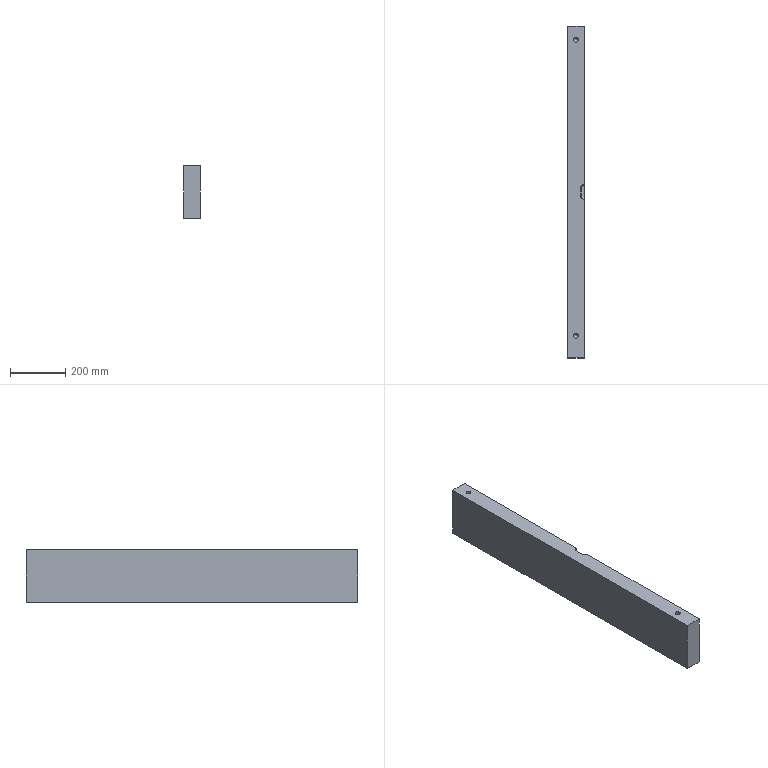Part | STEP file | lll_id4458_x_t | 1 solid | 25 faces | box 60 x 1200 x 190 mm | volume 13623980 mm3 | plane 10 | cylinder 9 | cone 4 | sphere 2 | commonest cylinder face diameters 20 x5 17.505 x2 17.506 x2
STEP:
#1=CARTESIAN_POINT('',(855.188,550.,-370.));
#2=VERTEX_POINT('',#1);
#3=CARTESIAN_POINT('',(846.435,550.,-370.));
#4=DIRECTION('',(0.,0.,1.));
#5=DIRECTION('',(1.,0.,0.));
#6=AXIS2_PLACEMENT_3D('',#3,#4,#5);
#7=CIRCLE('',#6,8.752);
#8=EDGE_CURVE('',#2,#2,#7,.T.);
#9=ORIENTED_EDGE('',*,*,#8,.T.);
#10=EDGE_LOOP('',(#9));
#11=FACE_BOUND('',#10,.T.);
#12=CARTESIAN_POINT('',(876.435,600.,-370.));
#13=VERTEX_POINT('',#12);
#14=CARTESIAN_POINT('',(876.435,-600.,-370.));
#15=VERTEX_POINT('',#14);
#16=CARTESIAN_POINT('',(876.435,600.,-370.));
#17=DIRECTION('',(0.,-1.,0.));
#18=VECTOR('',#17,1.);
#19=LINE('',#16,#18);
#20=EDGE_CURVE('',#13,#15,#19,.T.);
#21=ORIENTED_EDGE('',*,*,#20,.T.);
#22=CARTESIAN_POINT('',(816.435,-600.,-370.));
#23=VERTEX_POINT('',#22);
#24=CARTESIAN_POINT('',(876.435,-600.,-370.));
#25=DIRECTION('',(-1.,0.,0.));
#26=VECTOR('',#25,1.);
#27=LINE('',#24,#26);
#28=EDGE_CURVE('',#15,#23,#27,.T.);
#29=ORIENTED_EDGE('',*,*,#28,.T.);
#30=CARTESIAN_POINT('',(816.435,600.,-370.));
#31=VERTEX_POINT('',#30);
#32=CARTESIAN_POINT('',(816.435,1.,-370.));
#33=DIRECTION('',(0.,-1.,0.));
#34=VECTOR('',#33,1.);
#35=LINE('',#32,#34);
#36=EDGE_CURVE('',#31,#23,#35,.T.);
#37=ORIENTED_EDGE('',*,*,#36,.F.);
#38=CARTESIAN_POINT('',(-3093.565,600.,-370.));
#39=DIRECTION('',(1.,0.,0.));
#40=VECTOR('',#39,1.);
#41=LINE('',#38,#40);
#42=EDGE_CURVE('',#31,#13,#41,.T.);
#43=ORIENTED_EDGE('',*,*,#42,.T.);
#44=EDGE_LOOP('',(#21,#29,#37,#43));
#45=FACE_BOUND('',#44,.T.);
#46=CARTESIAN_POINT('',(855.188,-520.,-370.));
#47=VERTEX_POINT('',#46);
#48=CARTESIAN_POINT('',(846.435,-520.,-370.));
#49=DIRECTION('',(0.,0.,1.));
#50=DIRECTION('',(1.,0.,0.));
#51=AXIS2_PLACEMENT_3D('',#48,#49,#50);
#52=CIRCLE('',#51,8.752);
#53=EDGE_CURVE('',#47,#47,#52,.T.);
#54=ORIENTED_EDGE('',*,*,#53,.T.);
#55=EDGE_LOOP('',(#54));
#56=FACE_BOUND('',#55,.T.);
#57=CARTESIAN_POINT('',(3062.751,1.,-370.));
#58=DIRECTION('',(0.,0.,-1.));
#59=DIRECTION('',(-1.,0.,0.));
#60=AXIS2_PLACEMENT_3D('',#57,#58,#59);
#61=PLANE('',#60);
#62=ADVANCED_FACE('',(#11,#45,#56),#61,.T.);
#63=CARTESIAN_POINT('',(876.435,25.5,-180.));
#64=VERTEX_POINT('',#63);
#65=CARTESIAN_POINT('',(876.435,25.5,-194.289));
#66=VERTEX_POINT('',#65);
#67=CARTESIAN_POINT('',(876.435,25.5,-251.25));
#68=DIRECTION('',(0.,0.,-1.));
#69=VECTOR('',#68,1.);
#70=LINE('',#67,#69);
#71=EDGE_CURVE('',#64,#66,#70,.T.);
#72=ORIENTED_EDGE('',*,*,#71,.T.);
#73=CARTESIAN_POINT('',(876.435,15.5,-208.431));
#74=VERTEX_POINT('',#73);
#75=CARTESIAN_POINT('',(876.435,15.5,-194.289));
#76=DIRECTION('',(-1.,0.,0.));
#77=DIRECTION('',(0.,0.,1.));
#78=AXIS2_PLACEMENT_3D('',#75,#76,#77);
#79=ELLIPSE('',#78,14.142,10.);
#80=EDGE_CURVE('',#66,#74,#79,.T.);
#81=ORIENTED_EDGE('',*,*,#80,.T.);
#82=CARTESIAN_POINT('',(876.435,-15.5,-208.431));
#83=VERTEX_POINT('',#82);
#84=CARTESIAN_POINT('',(876.435,-204.288,-208.431));
#85=DIRECTION('',(0.,-1.,0.));
#86=VECTOR('',#85,1.);
#87=LINE('',#84,#86);
#88=EDGE_CURVE('',#74,#83,#87,.T.);
#89=ORIENTED_EDGE('',*,*,#88,.T.);
#90=CARTESIAN_POINT('',(876.435,-25.5,-194.289));
#91=VERTEX_POINT('',#90);
#92=CARTESIAN_POINT('',(876.435,-15.5,-194.289));
#93=DIRECTION('',(-1.,0.,0.));
#94=DIRECTION('',(0.,0.,-1.));
#95=AXIS2_PLACEMENT_3D('',#92,#93,#94);
#96=ELLIPSE('',#95,14.142,10.);
#97=EDGE_CURVE('',#83,#91,#96,.T.);
#98=ORIENTED_EDGE('',*,*,#97,.T.);
#99=CARTESIAN_POINT('',(876.435,-25.5,-180.));
#100=VERTEX_POINT('',#99);
#101=CARTESIAN_POINT('',(876.435,-25.5,-251.25));
#102=DIRECTION('',(0.,0.,1.));
#103=VECTOR('',#102,1.);
#104=LINE('',#101,#103);
#105=EDGE_CURVE('',#91,#100,#104,.T.);
#106=ORIENTED_EDGE('',*,*,#105,.T.);
#107=CARTESIAN_POINT('',(876.435,-600.,-180.));
#108=VERTEX_POINT('',#107);
#109=CARTESIAN_POINT('',(876.435,1.,-180.));
#110=DIRECTION('',(0.,-1.,0.));
#111=VECTOR('',#110,1.);
#112=LINE('',#109,#111);
#113=EDGE_CURVE('',#100,#108,#112,.T.);
#114=ORIENTED_EDGE('',*,*,#113,.T.);
#115=CARTESIAN_POINT('',(876.435,-600.,-182.5));
#116=DIRECTION('',(0.,0.,-1.));
#117=VECTOR('',#116,1.);
#118=LINE('',#115,#117);
#119=EDGE_CURVE('',#108,#15,#118,.T.);
#120=ORIENTED_EDGE('',*,*,#119,.T.);
#121=ORIENTED_EDGE('',*,*,#20,.F.);
#122=CARTESIAN_POINT('',(876.435,600.,-180.));
#123=VERTEX_POINT('',#122);
#124=CARTESIAN_POINT('',(876.435,600.,-182.5));
#125=DIRECTION('',(0.,0.,-1.));
#126=VECTOR('',#125,1.);
#127=LINE('',#124,#126);
#128=EDGE_CURVE('',#123,#13,#127,.T.);
#129=ORIENTED_EDGE('',*,*,#128,.F.);
#130=CARTESIAN_POINT('',(876.435,1.,-180.));
#131=DIRECTION('',(0.,-1.,0.));
#132=VECTOR('',#131,1.);
#133=LINE('',#130,#132);
#134=EDGE_CURVE('',#123,#64,#133,.T.);
#135=ORIENTED_EDGE('',*,*,#134,.T.);
#136=EDGE_LOOP('',(#72,#81,#89,#98,#106,#114,#120,#121,#129,#135));
#137=FACE_OUTER_BOUND('',#136,.T.);
#138=CARTESIAN_POINT('',(876.435,600.,-182.5));
#139=DIRECTION('',(1.,0.,0.));
#140=DIRECTION('',(0.,0.,-1.));
#141=AXIS2_PLACEMENT_3D('',#138,#139,#140);
#142=PLANE('',#141);
#143=ADVANCED_FACE('',(#137),#142,.T.);
#144=CARTESIAN_POINT('',(816.435,-600.,-180.));
#145=VERTEX_POINT('',#144);
#146=CARTESIAN_POINT('',(816.435,-600.,-182.5));
#147=DIRECTION('',(0.,0.,-1.));
#148=VECTOR('',#147,1.);
#149=LINE('',#146,#148);
#150=EDGE_CURVE('',#145,#23,#149,.T.);
#151=ORIENTED_EDGE('',*,*,#150,.T.);
#152=ORIENTED_EDGE('',*,*,#28,.F.);
#153=ORIENTED_EDGE('',*,*,#119,.F.);
#154=CARTESIAN_POINT('',(3062.751,-600.,-180.));
#155=DIRECTION('',(-1.,0.,0.));
#156=VECTOR('',#155,1.);
#157=LINE('',#154,#156);
#158=EDGE_CURVE('',#108,#145,#157,.T.);
#159=ORIENTED_EDGE('',*,*,#158,.T.);
#160=EDGE_LOOP('',(#151,#152,#153,#159));
#161=FACE_OUTER_BOUND('',#160,.T.);
#162=CARTESIAN_POINT('',(876.435,-600.,-182.5));
#163=DIRECTION('',(0.,-1.,0.));
#164=DIRECTION('',(0.,0.,-1.));
#165=AXIS2_PLACEMENT_3D('',#162,#163,#164);
#166=PLANE('',#165);
#167=ADVANCED_FACE('',(#161),#166,.T.);
#168=CARTESIAN_POINT('',(816.435,600.,-180.));
#169=VERTEX_POINT('',#168);
#170=CARTESIAN_POINT('',(816.435,600.,-182.5));
#171=DIRECTION('',(0.,0.,1.));
#172=VECTOR('',#171,1.);
#173=LINE('',#170,#172);
#174=EDGE_CURVE('',#31,#169,#173,.T.);
#175=ORIENTED_EDGE('',*,*,#174,.T.);
#176=CARTESIAN_POINT('',(3062.751,600.,-180.));
#177=DIRECTION('',(1.,0.,0.));
#178=VECTOR('',#177,1.);
#179=LINE('',#176,#178);
#180=EDGE_CURVE('',#169,#123,#179,.T.);
#181=ORIENTED_EDGE('',*,*,#180,.T.);
#182=ORIENTED_EDGE('',*,*,#128,.T.);
#183=ORIENTED_EDGE('',*,*,#42,.F.);
#184=EDGE_LOOP('',(#175,#181,#182,#183));
#185=FACE_OUTER_BOUND('',#184,.T.);
#186=CARTESIAN_POINT('',(-3093.565,600.,-182.5));
#187=DIRECTION('',(0.,1.,0.));
#188=DIRECTION('',(0.,0.,1.));
#189=AXIS2_PLACEMENT_3D('',#186,#187,#188);
#190=PLANE('',#189);
#191=ADVANCED_FACE('',(#185),#190,.T.);
#192=CARTESIAN_POINT('',(837.682,550.,-180.));
#193=VERTEX_POINT('',#192);
#194=CARTESIAN_POINT('',(846.435,550.,-180.));
#195=DIRECTION('',(0.,0.,-1.));
#196=DIRECTION('',(-1.,0.,0.));
#197=AXIS2_PLACEMENT_3D('',#194,#195,#196);
#198=CIRCLE('',#197,8.753);
#199=EDGE_CURVE('',#193,#193,#198,.T.);
#200=ORIENTED_EDGE('',*,*,#199,.T.);
#201=EDGE_LOOP('',(#200));
#202=FACE_BOUND('',#201,.T.);
#203=CARTESIAN_POINT('',(837.682,-520.,-180.));
#204=VERTEX_POINT('',#203);
#205=CARTESIAN_POINT('',(846.435,-520.,-180.));
#206=DIRECTION('',(0.,0.,-1.));
#207=DIRECTION('',(-1.,0.,0.));
#208=AXIS2_PLACEMENT_3D('',#205,#206,#207);
#209=CIRCLE('',#208,8.753);
#210=EDGE_CURVE('',#204,#204,#209,.T.);
#211=ORIENTED_EDGE('',*,*,#210,.T.);
#212=EDGE_LOOP('',(#211));
#213=FACE_BOUND('',#212,.T.);
#214=CARTESIAN_POINT('',(873.004,25.5,-180.));
#215=VERTEX_POINT('',#214);
#216=CARTESIAN_POINT('',(863.004,15.5,-180.));
#217=VERTEX_POINT('',#216);
#218=CARTESIAN_POINT('',(873.004,15.5,-180.));
#219=DIRECTION('',(0.,0.,1.));
#220=DIRECTION('',(1.,0.,0.));
#221=AXIS2_PLACEMENT_3D('',#218,#219,#220);
#222=CIRCLE('',#221,10.);
#223=EDGE_CURVE('',#215,#217,#222,.T.);
#224=ORIENTED_EDGE('',*,*,#223,.F.);
#225=CARTESIAN_POINT('',(898.504,25.5,-180.));
#226=DIRECTION('',(-1.,0.,0.));
#227=VECTOR('',#226,1.);
#228=LINE('',#225,#227);
#229=EDGE_CURVE('',#64,#215,#228,.T.);
#230=ORIENTED_EDGE('',*,*,#229,.F.);
#231=ORIENTED_EDGE('',*,*,#134,.F.);
#232=ORIENTED_EDGE('',*,*,#180,.F.);
#233=CARTESIAN_POINT('',(816.435,0.,-180.));
#234=DIRECTION('',(0.,1.,0.));
#235=VECTOR('',#234,1.);
#236=LINE('',#233,#235);
#237=EDGE_CURVE('',#145,#169,#236,.T.);
#238=ORIENTED_EDGE('',*,*,#237,.F.);
#239=ORIENTED_EDGE('',*,*,#158,.F.);
#240=ORIENTED_EDGE('',*,*,#113,.F.);
#241=CARTESIAN_POINT('',(873.004,-25.5,-180.));
#242=VERTEX_POINT('',#241);
#243=CARTESIAN_POINT('',(898.504,-25.5,-180.));
#244=DIRECTION('',(1.,0.,0.));
#245=VECTOR('',#244,1.);
#246=LINE('',#243,#245);
#247=EDGE_CURVE('',#242,#100,#246,.T.);
#248=ORIENTED_EDGE('',*,*,#247,.F.);
#249=CARTESIAN_POINT('',(863.004,-15.5,-180.));
#250=VERTEX_POINT('',#249);
#251=CARTESIAN_POINT('',(873.004,-15.5,-180.));
#252=DIRECTION('',(0.,0.,1.));
#253=DIRECTION('',(1.,0.,0.));
#254=AXIS2_PLACEMENT_3D('',#251,#252,#253);
#255=CIRCLE('',#254,10.);
#256=EDGE_CURVE('',#250,#242,#255,.T.);
#257=ORIENTED_EDGE('',*,*,#256,.F.);
#258=CARTESIAN_POINT('',(863.004,0.,-180.));
#259=DIRECTION('',(0.,-1.,0.));
#260=VECTOR('',#259,1.);
#261=LINE('',#258,#260);
#262=EDGE_CURVE('',#217,#250,#261,.T.);
#263=ORIENTED_EDGE('',*,*,#262,.F.);
#264=EDGE_LOOP('',(#224,#230,#231,#232,#238,#239,#240,#248,#257,#263));
#265=FACE_BOUND('',#264,.T.);
#266=CARTESIAN_POINT('',(3062.751,1.,-180.));
#267=DIRECTION('',(0.,0.,-1.));
#268=DIRECTION('',(-1.,0.,0.));
#269=AXIS2_PLACEMENT_3D('',#266,#267,#268);
#270=PLANE('',#269);
#271=ADVANCED_FACE('',(#202,#213,#265),#270,.F.);
#272=ORIENTED_EDGE('',*,*,#174,.F.);
#273=ORIENTED_EDGE('',*,*,#36,.T.);
#274=ORIENTED_EDGE('',*,*,#150,.F.);
#275=ORIENTED_EDGE('',*,*,#237,.T.);
#276=EDGE_LOOP('',(#272,#273,#274,#275));
#277=FACE_OUTER_BOUND('',#276,.T.);
#278=CARTESIAN_POINT('',(816.435,0.,-251.25));
#279=DIRECTION('',(1.,0.,0.));
#280=DIRECTION('',(0.,0.,-1.));
#281=AXIS2_PLACEMENT_3D('',#278,#279,#280);
#282=PLANE('',#281);
#283=ADVANCED_FACE('',(#277),#282,.F.);
#284=ORIENTED_EDGE('',*,*,#88,.F.);
#285=CARTESIAN_POINT('',(865.933,15.5,-197.929));
#286=VERTEX_POINT('',#285);
#287=CARTESIAN_POINT('',(876.435,15.5,-208.431));
#288=DIRECTION('',(0.7071,0.,-0.7071));
#289=VECTOR('',#288,1.);
#290=LINE('',#287,#289);
#291=EDGE_CURVE('',#286,#74,#290,.T.);
#292=ORIENTED_EDGE('',*,*,#291,.F.);
#293=CARTESIAN_POINT('',(865.933,-15.5,-197.929));
#294=VERTEX_POINT('',#293);
#295=CARTESIAN_POINT('',(865.933,35.5,-197.929));
#296=DIRECTION('',(0.,1.,0.));
#297=VECTOR('',#296,1.);
#298=LINE('',#295,#297);
#299=EDGE_CURVE('',#294,#286,#298,.T.);
#300=ORIENTED_EDGE('',*,*,#299,.F.);
#301=CARTESIAN_POINT('',(863.004,-15.5,-195.));
#302=DIRECTION('',(-0.7071,0.,0.7071));
#303=VECTOR('',#302,1.);
#304=LINE('',#301,#303);
#305=EDGE_CURVE('',#83,#294,#304,.T.);
#306=ORIENTED_EDGE('',*,*,#305,.F.);
#307=EDGE_LOOP('',(#284,#292,#300,#306));
#308=FACE_OUTER_BOUND('',#307,.T.);
#309=CARTESIAN_POINT('',(863.004,0.,-195.));
#310=DIRECTION('',(0.7071,0.,0.7071));
#311=DIRECTION('',(0.,1.,0.));
#312=AXIS2_PLACEMENT_3D('',#309,#310,#311);
#313=PLANE('',#312);
#314=ADVANCED_FACE('',(#308),#313,.T.);
#315=ORIENTED_EDGE('',*,*,#223,.T.);
#316=CARTESIAN_POINT('',(863.004,15.5,-190.858));
#317=VERTEX_POINT('',#316);
#318=CARTESIAN_POINT('',(863.004,15.5,-195.));
#319=DIRECTION('',(0.,0.,-1.));
#320=VECTOR('',#319,1.);
#321=LINE('',#318,#320);
#322=EDGE_CURVE('',#217,#317,#321,.T.);
#323=ORIENTED_EDGE('',*,*,#322,.T.);
#324=CARTESIAN_POINT('',(873.004,25.5,-190.858));
#325=VERTEX_POINT('',#324);
#326=CARTESIAN_POINT('',(873.004,15.5,-190.858));
#327=DIRECTION('',(0.,0.,-1.));
#328=DIRECTION('',(-1.,0.,0.));
#329=AXIS2_PLACEMENT_3D('',#326,#327,#328);
#330=CIRCLE('',#329,10.);
#331=EDGE_CURVE('',#317,#325,#330,.T.);
#332=ORIENTED_EDGE('',*,*,#331,.T.);
#333=CARTESIAN_POINT('',(873.004,25.5,-180.));
#334=DIRECTION('',(0.,0.,1.));
#335=VECTOR('',#334,1.);
#336=LINE('',#333,#335);
#337=EDGE_CURVE('',#325,#215,#336,.T.);
#338=ORIENTED_EDGE('',*,*,#337,.T.);
#339=EDGE_LOOP('',(#315,#323,#332,#338));
#340=FACE_OUTER_BOUND('',#339,.T.);
#341=CARTESIAN_POINT('',(873.004,15.5,-210.));
#342=DIRECTION('',(0.,0.,1.));
#343=DIRECTION('',(-1.,0.,0.));
#344=AXIS2_PLACEMENT_3D('',#341,#342,#343);
#345=CYLINDRICAL_SURFACE('',#344,10.);
#346=ADVANCED_FACE('',(#340),#345,.F.);
#347=ORIENTED_EDGE('',*,*,#80,.F.);
#348=CARTESIAN_POINT('',(870.075,25.5,-187.929));
#349=DIRECTION('',(-0.7071,0.,0.7071));
#350=VECTOR('',#349,1.);
#351=LINE('',#348,#350);
#352=EDGE_CURVE('',#66,#325,#351,.T.);
#353=ORIENTED_EDGE('',*,*,#352,.T.);
#354=CARTESIAN_POINT('',(873.004,15.5,-190.858));
#355=DIRECTION('',(-0.7071,0.,0.7071));
#356=DIRECTION('',(-0.7071,0.,-0.7071));
#357=AXIS2_PLACEMENT_3D('',#354,#355,#356);
#358=CIRCLE('',#357,10.);
#359=EDGE_CURVE('',#325,#286,#358,.T.);
#360=ORIENTED_EDGE('',*,*,#359,.T.);
#361=ORIENTED_EDGE('',*,*,#291,.T.);
#362=EDGE_LOOP('',(#347,#353,#360,#361));
#363=FACE_OUTER_BOUND('',#362,.T.);
#364=CARTESIAN_POINT('',(895.325,15.5,-213.179));
#365=DIRECTION('',(-0.7071,0.,0.7071));
#366=DIRECTION('',(-0.7071,0.,-0.7071));
#367=AXIS2_PLACEMENT_3D('',#364,#365,#366);
#368=CYLINDRICAL_SURFACE('',#367,10.);
#369=ADVANCED_FACE('',(#363),#368,.F.);
#370=CARTESIAN_POINT('',(873.004,15.5,-190.858));
#371=DIRECTION('',(0.,-1.,0.));
#372=DIRECTION('',(0.,0.,-1.));
#373=AXIS2_PLACEMENT_3D('',#370,#371,#372);
#374=CIRCLE('',#373,10.);
#375=EDGE_CURVE('',#317,#286,#374,.T.);
#376=ORIENTED_EDGE('',*,*,#375,.F.);
#377=CARTESIAN_POINT('',(863.004,-15.5,-190.858));
#378=VERTEX_POINT('',#377);
#379=CARTESIAN_POINT('',(863.004,-35.5,-190.858));
#380=DIRECTION('',(0.,-1.,0.));
#381=VECTOR('',#380,1.);
#382=LINE('',#379,#381);
#383=EDGE_CURVE('',#317,#378,#382,.T.);
#384=ORIENTED_EDGE('',*,*,#383,.T.);
#385=CARTESIAN_POINT('',(873.004,-15.5,-190.858));
#386=DIRECTION('',(0.,-1.,0.));
#387=DIRECTION('',(0.,0.,-1.));
#388=AXIS2_PLACEMENT_3D('',#385,#386,#387);
#389=CIRCLE('',#388,10.);
#390=EDGE_CURVE('',#378,#294,#389,.T.);
#391=ORIENTED_EDGE('',*,*,#390,.T.);
#392=ORIENTED_EDGE('',*,*,#299,.T.);
#393=EDGE_LOOP('',(#376,#384,#391,#392));
#394=FACE_OUTER_BOUND('',#393,.T.);
#395=CARTESIAN_POINT('',(873.004,0.,-190.858));
#396=DIRECTION('',(0.,-1.,0.));
#397=DIRECTION('',(0.,0.,-1.));
#398=AXIS2_PLACEMENT_3D('',#395,#396,#397);
#399=CYLINDRICAL_SURFACE('',#398,10.);
#400=ADVANCED_FACE('',(#394),#399,.F.);
#401=ORIENTED_EDGE('',*,*,#331,.F.);
#402=ORIENTED_EDGE('',*,*,#375,.T.);
#403=ORIENTED_EDGE('',*,*,#359,.F.);
#404=EDGE_LOOP('',(#401,#402,#403));
#405=FACE_OUTER_BOUND('',#404,.T.);
#406=CARTESIAN_POINT('',(873.004,15.5,-190.858));
#407=DIRECTION('',(0.,0.,1.));
#408=DIRECTION('',(-1.,0.,0.));
#409=AXIS2_PLACEMENT_3D('',#406,#407,#408);
#410=SPHERICAL_SURFACE('',#409,10.);
#411=ADVANCED_FACE('',(#405),#410,.F.);
#412=ORIENTED_EDGE('',*,*,#256,.T.);
#413=CARTESIAN_POINT('',(873.004,-25.5,-190.858));
#414=VERTEX_POINT('',#413);
#415=CARTESIAN_POINT('',(873.004,-25.5,-195.));
#416=DIRECTION('',(0.,0.,-1.));
#417=VECTOR('',#416,1.);
#418=LINE('',#415,#417);
#419=EDGE_CURVE('',#242,#414,#418,.T.);
#420=ORIENTED_EDGE('',*,*,#419,.T.);
#421=CARTESIAN_POINT('',(873.004,-15.5,-190.858));
#422=DIRECTION('',(0.,0.,-1.));
#423=DIRECTION('',(-1.,0.,0.));
#424=AXIS2_PLACEMENT_3D('',#421,#422,#423);
#425=CIRCLE('',#424,10.);
#426=EDGE_CURVE('',#414,#378,#425,.T.);
#427=ORIENTED_EDGE('',*,*,#426,.T.);
#428=CARTESIAN_POINT('',(863.004,-15.5,-180.));
#429=DIRECTION('',(0.,0.,1.));
#430=VECTOR('',#429,1.);
#431=LINE('',#428,#430);
#432=EDGE_CURVE('',#378,#250,#431,.T.);
#433=ORIENTED_EDGE('',*,*,#432,.T.);
#434=EDGE_LOOP('',(#412,#420,#427,#433));
#435=FACE_OUTER_BOUND('',#434,.T.);
#436=CARTESIAN_POINT('',(873.004,-15.5,-210.));
#437=DIRECTION('',(0.,0.,1.));
#438=DIRECTION('',(-1.,0.,0.));
#439=AXIS2_PLACEMENT_3D('',#436,#437,#438);
#440=CYLINDRICAL_SURFACE('',#439,10.);
#441=ADVANCED_FACE('',(#435),#440,.F.);
#442=ORIENTED_EDGE('',*,*,#426,.F.);
#443=CARTESIAN_POINT('',(873.004,-15.5,-190.858));
#444=DIRECTION('',(0.7071,0.,-0.7071));
#445=DIRECTION('',(0.7071,0.,0.7071));
#446=AXIS2_PLACEMENT_3D('',#443,#444,#445);
#447=CIRCLE('',#446,10.);
#448=EDGE_CURVE('',#414,#294,#447,.T.);
#449=ORIENTED_EDGE('',*,*,#448,.T.);
#450=ORIENTED_EDGE('',*,*,#390,.F.);
#451=EDGE_LOOP('',(#442,#449,#450));
#452=FACE_OUTER_BOUND('',#451,.T.);
#453=CARTESIAN_POINT('',(873.004,-15.5,-190.858));
#454=DIRECTION('',(0.,0.,1.));
#455=DIRECTION('',(-1.,0.,0.));
#456=AXIS2_PLACEMENT_3D('',#453,#454,#455);
#457=SPHERICAL_SURFACE('',#456,10.);
#458=ADVANCED_FACE('',(#452),#457,.F.);
#459=ORIENTED_EDGE('',*,*,#448,.F.);
#460=CARTESIAN_POINT('',(883.506,-25.5,-201.36));
#461=DIRECTION('',(0.7071,0.,-0.7071));
#462=VECTOR('',#461,1.);
#463=LINE('',#460,#462);
#464=EDGE_CURVE('',#414,#91,#463,.T.);
#465=ORIENTED_EDGE('',*,*,#464,.T.);
#466=ORIENTED_EDGE('',*,*,#97,.F.);
#467=ORIENTED_EDGE('',*,*,#305,.T.);
#468=EDGE_LOOP('',(#459,#465,#466,#467));
#469=FACE_OUTER_BOUND('',#468,.T.);
#470=CARTESIAN_POINT('',(895.325,-15.5,-213.179));
#471=DIRECTION('',(0.7071,0.,-0.7071));
#472=DIRECTION('',(0.7071,0.,0.7071));
#473=AXIS2_PLACEMENT_3D('',#470,#471,#472);
#474=CYLINDRICAL_SURFACE('',#473,10.);
#475=ADVANCED_FACE('',(#469),#474,.F.);
#476=ORIENTED_EDGE('',*,*,#352,.F.);
#477=ORIENTED_EDGE('',*,*,#71,.F.);
#478=ORIENTED_EDGE('',*,*,#229,.T.);
#479=ORIENTED_EDGE('',*,*,#337,.F.);
#480=EDGE_LOOP('',(#476,#477,#478,#479));
#481=FACE_OUTER_BOUND('',#480,.T.);
#482=CARTESIAN_POINT('',(898.504,25.5,-210.));
#483=DIRECTION('',(0.,1.,0.));
#484=DIRECTION('',(0.,0.,1.));
#485=AXIS2_PLACEMENT_3D('',#482,#483,#484);
#486=PLANE('',#485);
#487=ADVANCED_FACE('',(#481),#486,.F.);
#488=ORIENTED_EDGE('',*,*,#419,.F.);
#489=ORIENTED_EDGE('',*,*,#247,.T.);
#490=ORIENTED_EDGE('',*,*,#105,.F.);
#491=ORIENTED_EDGE('',*,*,#464,.F.);
#492=EDGE_LOOP('',(#488,#489,#490,#491));
#493=FACE_OUTER_BOUND('',#492,.T.);
#494=CARTESIAN_POINT('',(898.504,-25.5,-210.));
#495=DIRECTION('',(0.,-1.,0.));
#496=DIRECTION('',(0.,0.,-1.));
#497=AXIS2_PLACEMENT_3D('',#494,#495,#496);
#498=PLANE('',#497);
#499=ADVANCED_FACE('',(#493),#498,.F.);
#500=ORIENTED_EDGE('',*,*,#383,.F.);
#501=ORIENTED_EDGE('',*,*,#322,.F.);
#502=ORIENTED_EDGE('',*,*,#262,.T.);
#503=ORIENTED_EDGE('',*,*,#432,.F.);
#504=EDGE_LOOP('',(#500,#501,#502,#503));
#505=FACE_OUTER_BOUND('',#504,.T.);
#506=CARTESIAN_POINT('',(863.004,0.,-210.));
#507=DIRECTION('',(-1.,0.,0.));
#508=DIRECTION('',(0.,0.,-1.));
#509=AXIS2_PLACEMENT_3D('',#506,#507,#508);
#510=PLANE('',#509);
#511=ADVANCED_FACE('',(#505),#510,.F.);
#512=CARTESIAN_POINT('',(855.188,550.,-328.747));
#513=VERTEX_POINT('',#512);
#514=CARTESIAN_POINT('',(846.435,550.,-328.747));
#515=DIRECTION('',(0.,0.,1.));
#516=DIRECTION('',(1.,0.,0.));
#517=AXIS2_PLACEMENT_3D('',#514,#515,#516);
#518=CIRCLE('',#517,8.752);
#519=EDGE_CURVE('',#513,#513,#518,.T.);
#520=ORIENTED_EDGE('',*,*,#519,.T.);
#521=EDGE_LOOP('',(#520));
#522=FACE_BOUND('',#521,.T.);
#523=ORIENTED_EDGE('',*,*,#8,.F.);
#524=EDGE_LOOP('',(#523));
#525=FACE_BOUND('',#524,.T.);
#526=CARTESIAN_POINT('',(846.435,550.,-370.));
#527=DIRECTION('',(0.,0.,1.));
#528=DIRECTION('',(-1.,0.,0.));
#529=AXIS2_PLACEMENT_3D('',#526,#527,#528);
#530=CYLINDRICAL_SURFACE('',#529,8.752);
#531=ADVANCED_FACE('',(#522,#525),#530,.F.);
#532=CARTESIAN_POINT('',(846.435,550.,-319.994));
#533=VERTEX_POINT('',#532);
#534=VERTEX_LOOP('',#533);
#535=FACE_BOUND('',#534,.T.);
#536=ORIENTED_EDGE('',*,*,#519,.F.);
#537=EDGE_LOOP('',(#536));
#538=FACE_BOUND('',#537,.T.);
#539=CARTESIAN_POINT('',(846.435,550.,-328.747));
#540=DIRECTION('',(0.,0.,-1.));
#541=DIRECTION('',(1.,0.,0.));
#542=AXIS2_PLACEMENT_3D('',#539,#540,#541);
#543=CONICAL_SURFACE('',#542,8.752,45.);
#544=ADVANCED_FACE('',(#535,#538),#543,.F.);
#545=CARTESIAN_POINT('',(855.188,-520.,-328.747));
#546=VERTEX_POINT('',#545);
#547=CARTESIAN_POINT('',(846.435,-520.,-328.747));
#548=DIRECTION('',(0.,0.,1.));
#549=DIRECTION('',(1.,0.,0.));
#550=AXIS2_PLACEMENT_3D('',#547,#548,#549);
#551=CIRCLE('',#550,8.752);
#552=EDGE_CURVE('',#546,#546,#551,.T.);
#553=ORIENTED_EDGE('',*,*,#552,.T.);
#554=EDGE_LOOP('',(#553));
#555=FACE_BOUND('',#554,.T.);
#556=ORIENTED_EDGE('',*,*,#53,.F.);
#557=EDGE_LOOP('',(#556));
#558=FACE_BOUND('',#557,.T.);
#559=CARTESIAN_POINT('',(846.435,-520.,-370.));
#560=DIRECTION('',(0.,0.,1.));
#561=DIRECTION('',(-1.,0.,0.));
#562=AXIS2_PLACEMENT_3D('',#559,#560,#561);
#563=CYLINDRICAL_SURFACE('',#562,8.752);
#564=ADVANCED_FACE('',(#555,#558),#563,.F.);
#565=CARTESIAN_POINT('',(846.435,-520.,-319.994));
#566=VERTEX_POINT('',#565);
#567=VERTEX_LOOP('',#566);
#568=FACE_BOUND('',#567,.T.);
#569=ORIENTED_EDGE('',*,*,#552,.F.);
#570=EDGE_LOOP('',(#569));
#571=FACE_BOUND('',#570,.T.);
#572=CARTESIAN_POINT('',(846.435,-520.,-328.747));
#573=DIRECTION('',(0.,0.,-1.));
#574=DIRECTION('',(1.,0.,0.));
#575=AXIS2_PLACEMENT_3D('',#572,#573,#574);
#576=CONICAL_SURFACE('',#575,8.752,45.);
#577=ADVANCED_FACE('',(#568,#571),#576,.F.);
#578=CARTESIAN_POINT('',(837.682,-520.,-221.253));
#579=VERTEX_POINT('',#578);
#580=CARTESIAN_POINT('',(846.435,-520.,-221.253));
#581=DIRECTION('',(0.,0.,-1.));
#582=DIRECTION('',(-1.,0.,0.));
#583=AXIS2_PLACEMENT_3D('',#580,#581,#582);
#584=CIRCLE('',#583,8.753);
#585=EDGE_CURVE('',#579,#579,#584,.T.);
#586=ORIENTED_EDGE('',*,*,#585,.T.);
#587=EDGE_LOOP('',(#586));
#588=FACE_BOUND('',#587,.T.);
#589=ORIENTED_EDGE('',*,*,#210,.F.);
#590=EDGE_LOOP('',(#589));
#591=FACE_BOUND('',#590,.T.);
#592=CARTESIAN_POINT('',(846.435,-520.,-180.));
#593=DIRECTION('',(0.,0.,-1.));
#594=DIRECTION('',(1.,0.,0.));
#595=AXIS2_PLACEMENT_3D('',#592,#593,#594);
#596=CYLINDRICAL_SURFACE('',#595,8.753);
#597=ADVANCED_FACE('',(#588,#591),#596,.F.);
#598=CARTESIAN_POINT('',(846.435,-520.,-230.006));
#599=VERTEX_POINT('',#598);
#600=VERTEX_LOOP('',#599);
#601=FACE_BOUND('',#600,.T.);
#602=ORIENTED_EDGE('',*,*,#585,.F.);
#603=EDGE_LOOP('',(#602));
#604=FACE_BOUND('',#603,.T.);
#605=CARTESIAN_POINT('',(846.435,-520.,-221.253));
#606=DIRECTION('',(0.,0.,1.));
#607=DIRECTION('',(-1.,0.,0.));
#608=AXIS2_PLACEMENT_3D('',#605,#606,#607);
#609=CONICAL_SURFACE('',#608,8.753,45.);
#610=ADVANCED_FACE('',(#601,#604),#609,.F.);
#611=CARTESIAN_POINT('',(837.682,550.,-221.253));
#612=VERTEX_POINT('',#611);
#613=CARTESIAN_POINT('',(846.435,550.,-221.253));
#614=DIRECTION('',(0.,0.,-1.));
#615=DIRECTION('',(-1.,0.,0.));
#616=AXIS2_PLACEMENT_3D('',#613,#614,#615);
#617=CIRCLE('',#616,8.753);
#618=EDGE_CURVE('',#612,#612,#617,.T.);
#619=ORIENTED_EDGE('',*,*,#618,.T.);
#620=EDGE_LOOP('',(#619));
#621=FACE_BOUND('',#620,.T.);
#622=ORIENTED_EDGE('',*,*,#199,.F.);
#623=EDGE_LOOP('',(#622));
#624=FACE_BOUND('',#623,.T.);
#625=CARTESIAN_POINT('',(846.435,550.,-180.));
#626=DIRECTION('',(0.,0.,-1.));
#627=DIRECTION('',(1.,0.,0.));
#628=AXIS2_PLACEMENT_3D('',#625,#626,#627);
#629=CYLINDRICAL_SURFACE('',#628,8.753);
#630=ADVANCED_FACE('',(#621,#624),#629,.F.);
#631=CARTESIAN_POINT('',(846.435,550.,-230.006));
#632=VERTEX_POINT('',#631);
#633=VERTEX_LOOP('',#632);
#634=FACE_BOUND('',#633,.T.);
#635=ORIENTED_EDGE('',*,*,#618,.F.);
#636=EDGE_LOOP('',(#635));
#637=FACE_BOUND('',#636,.T.);
#638=CARTESIAN_POINT('',(846.435,550.,-221.253));
#639=DIRECTION('',(0.,0.,1.));
#640=DIRECTION('',(-1.,0.,0.));
#641=AXIS2_PLACEMENT_3D('',#638,#639,#640);
#642=CONICAL_SURFACE('',#641,8.753,45.);
#643=ADVANCED_FACE('',(#634,#637),#642,.F.);
#644=CLOSED_SHELL('',(#62,#143,#167,#191,#271,#283,#314,#346,#369,#400,#411,#441,#458,#475,#487,#499,#511,#531,#544,#564,#577,#597,#610,#630,#643));
#645=MANIFOLD_SOLID_BREP('',#644);
#646=(LENGTH_UNIT()NAMED_UNIT(*)SI_UNIT(.MILLI.,.METRE.));
#647=UNCERTAINTY_MEASURE_WITH_UNIT(LENGTH_MEASURE(0.00002),#646,'','');
#648=(NAMED_UNIT(*)PLANE_ANGLE_UNIT()SI_UNIT($,.RADIAN.));
#649=PLANE_ANGLE_MEASURE_WITH_UNIT(PLANE_ANGLE_MEASURE(0.01745),#648);
#650=DIMENSIONAL_EXPONENTS(0.,0.,0.,0.,0.,0.,0.);
#651=(CONVERSION_BASED_UNIT('DEGREE',#649)NAMED_UNIT(#650)PLANE_ANGLE_UNIT());
#652=(NAMED_UNIT(*)SI_UNIT($,.STERADIAN.)SOLID_ANGLE_UNIT());
#653=(GEOMETRIC_REPRESENTATION_CONTEXT(3)GLOBAL_UNCERTAINTY_ASSIGNED_CONTEXT((#647))GLOBAL_UNIT_ASSIGNED_CONTEXT((#646,#651,#652))REPRESENTATION_CONTEXT('',''));
#654=ADVANCED_BREP_SHAPE_REPRESENTATION('',(#645),#653);